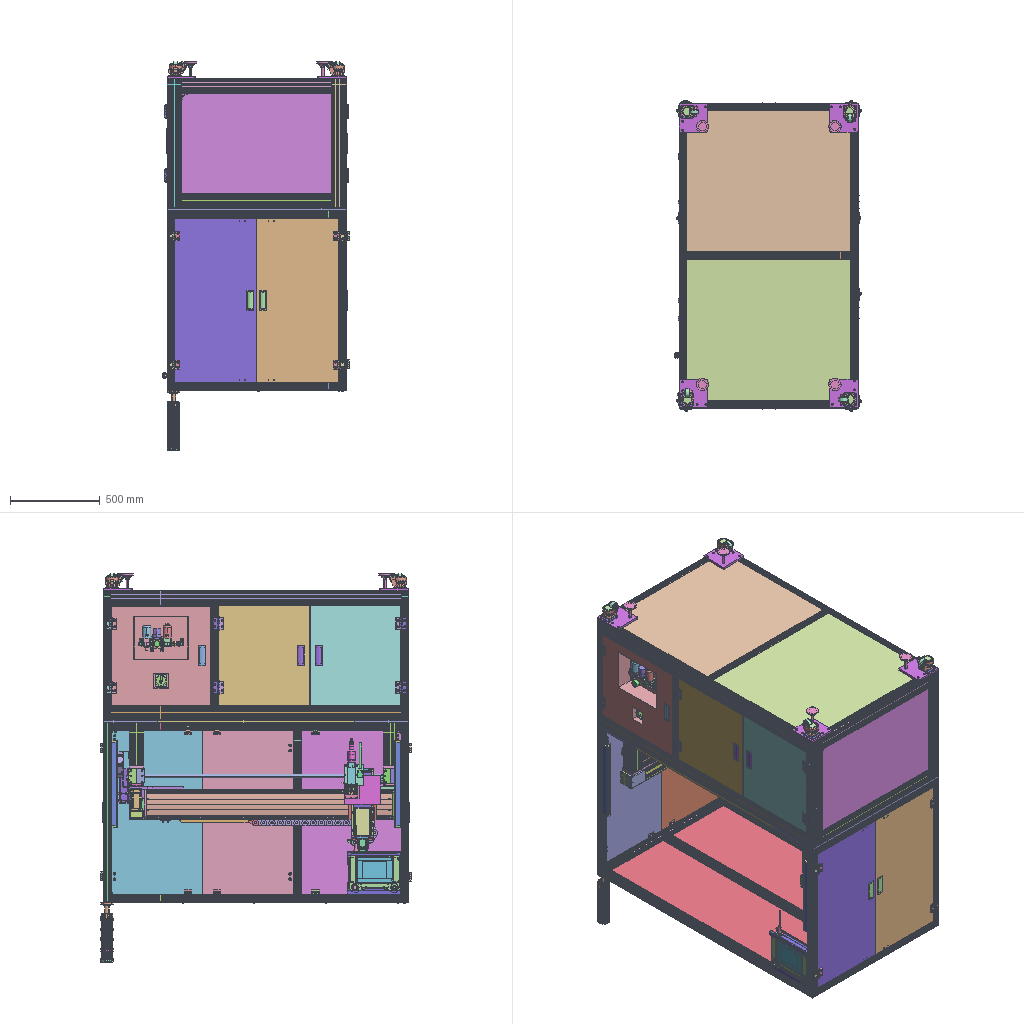Assembly | STEP file | 300 different items | 915 placed | box 1041 x 1735 x 2168 mm
Parts list (item | name | quantity | parent item | size | volume):
1 | 10B | x1 | in 20201224-195616-35202 | 290 x 230 x 35 mm | 178188 mm3
2 | 11B | x1 | in 20201224-195616-35202 | 290 x 385 x 37.5 mm | 218260 mm3
3 | 11M | x1 | in PLASMA | 71 x 79.5 x 170.1 mm | 187590 mm3
4 | 2 reset flat push button[GOB-2A10M-GW]_10M | x1 | in 2 reset flat push button[GOB-2A10M-GW]_GOB-2A10M-GW | 71 x 79.5 x 130.1 mm | 149787 mm3
5 | 82 fan grille | x1 | in Power supply model--JYDM(2)1 | 124.466 x 2.25 x 124.466 mm | 2127 mm3
6 | AC220V three-pin socket-KET-301 | x1 | in Power supply model--JYDM(2)1 | 50.485 x 22.8 x 28.4 mm | 5143 mm3
7 | AIR_PRESSURE_REGULATOR_SCREEN | x1 | in Power supply model--JYDM(2)1 | - | -
8 | AP0_ASM_ALL_SHEET_09 | x1 | in APO_ASM_SHEET_JYDM_WELDING_ASM | - | -
9 | AP0_ASM_ALL_SHEET_10 | x1 | in APO_ASM_SHEET_JYDM_WELDING_ASM | - | -
10 | AP0_ASM_ALL_SHEET_11 | x1 | in APO_ASM_SHEET_JYDM_WELDING_ASM | - | -
11 | AP0_ASM_JYDM_SHEET_04 | x1 | in Power supply model--JYDM(2)1 | 396.5 x 248 x 20 mm | 232744 mm3
12 | AP0_JYDM_SHEET_01 | x1 | in APO_ASM_SHEET_JYDM_WELDING_ASM | - | -
13 | AP0_JYDM_SHEET_02_05 | x1 | in APO_ASM_SHEET_JYDM_WELDING_ASM | - | -
14 | AP0_JYDM_SHEET_03 | x1 | in APO_ASM_SHEET_JYDM_WELDING_ASM | - | -
15 | AP0_JYDM_SHEET_07 | x1 | in Power supply model--JYDM(2)1 | 58 x 58 x 27.5 mm | 7319 mm3
16 | AP0_JYDM_SHEET_15 | x2 | in APO_ASM_SHEET_JYDM_WELDING_ASM | 20 x 13.5 x 70 mm | 4064 mm3
17 | B01-_X2_70B980F6_X0_ | x1 | in Standard three-color light | 68.5 x 68.5 x 39.5 mm | 31380 mm3
18 | Black terminal post | x1 | in Power supply model--JYDM(2)1 | 20.458 x 20.454 x 38 mm | 10782 mm3
19 | Blowing port | x1 | in Function head assembly | 19 x 192 x 30 mm | 38106 mm3
20 | CNTG-8 | x3 | in Power supply model--JYDM(2)1 | 38 x 22.2 x 22.2 mm | 6916 mm3
21 | Changeover switch LW30-63.... | x1 | in HJC0 frame | 65 x 65 x 101.647 mm | 216311 mm3
22 | FFH80-GY-002A^FFH85-B3 -02_three-axis module | x1 | in FFH85-B3 -02^three-axis module | 110 x 81 x 42.5 mm | 368601 mm3
23 | FFH80-GY-002A^FFH85-PL-M75-B3-01_three-axis module | x1 | in FFH85-PL-M75-B3-01^three-axis module | 110 x 81 x 42.5 mm | 368601 mm3
24 | FFH80-GY-002B^FFH85-B3 -02_three-axis module | x1 | in FFH85-B3 -02^three-axis module | 110 x 81 x 42.5 mm | 366642 mm3
25 | FFH80-GY-002B^FFH85-PL-M75-B3-01_three-axis module | x1 | in FFH85-PL-M75-B3-01^three-axis module | 110 x 81 x 42.5 mm | 366642 mm3
26 | FFH80-GY-003A^FFH85-PL-M75-B3-01_three-axis module | x1 | in FFH85-PL-M75-B3-01^three-axis module | 90 x 81 x 42.5 mm | 300723 mm3
27 | FFH80-GY-003B^FFH85-B3 -02_three-axis module | x1 | in FFH85-B3 -02^three-axis module | 90 x 81 x 42.5 mm | 303054 mm3
28 | FFH80-GY-003B^FFH85-PL-M75-B3-01_three-axis module | x1 | in FFH85-PL-M75-B3-01^three-axis module | 90 x 81 x 42.5 mm | 303221 mm3
29 | FFH80-GY-004^FFH85-B3 -02_three-axis module | x1 | in FFH85-B3 -02^three-axis module | 78 x 17.5 x 210 mm | 184560 mm3
30 | FFH80-GY-004^FFH85-PL-M75-B3-01_three-axis module | x1 | in FFH85-PL-M75-B3-01^three-axis module | 78 x 17.5 x 210 mm | 184560 mm3
31 | FFH80-GY-007^FFH85-PL-M75-B3-01_three-axis module | x1 | in FFH85-PL-M75-B3-01^three-axis module | 16.7 x 71.8 x 210 mm | 16698 mm3
32 | FFH80-GY-019^FFH85-B3 -02_three-axis module | x1 | in FFH85-B3 -02^three-axis module | 11 x 32.5 x 30 mm | 540.052 mm3
33 | FFH80-GY-020^FFH85-B3 -02_three-axis module | x1 | in FFH85-B3 -02^three-axis module | 1 x 12 x 52 mm | 601.324 mm3
34 | FFH80-GY-020^FFH85-PL-M75-B3-01_three-axis module | x1 | in FFH85-PL-M75-B3-01^three-axis module | 1 x 12 x 52 mm | 601.324 mm3
35 | FFH80-GY-022^FFH85-B3 -02_three-axis module | x1 | in FFH85-B3 -02^three-axis module | 1 x 60 x 60 mm | 3497 mm3
36 | FFH80-GY-022^FFH85-PL-M75-B3-01_three-axis module | x1 | in FFH85-PL-M75-B3-01^three-axis module | 1 x 60 x 60 mm | 3183 mm3
37 | FFH80-PL-008^FFH85-PL-M75-B3-01_three-axis module | x1 | in FFH85-PL-M75-B3-01^three-axis module | 10 x 81 x 192 mm | 99409 mm3
38 | FFH80-PL-018^FFH85-PL-M75-B3-01_three-axis module | x1 | in FFH85-PL-M75-B3-01^three-axis module | 40 x 81 x 192 mm | 36491 mm3
39 | FFH85-PL-011^FFH85-B3 -02_three-axis module | x1 | in FFH85-B3 -02^three-axis module | 85 x 81.5 x 722 mm | 4571503 mm3
40 | FFH85-PL-011^FFH85-PL-M75-B3-01_three-axis module | x1 | in FFH85-PL-M75-B3-01^three-axis module | 85 x 81.5 x 722 mm | 4571503 mm3
41 | LES120 base^FTH120-PD-direct-drive motor | x1 | in FTH120-PD-direct-drive motor | 120 x 58.2 x 361 mm | 888323 mm3
42 | LES120 bearing housing^FTH120-PD-direct-drive motor | x1 | in FTH120-PD-direct-drive motor | 119 x 56.7 x 13 mm | 72115 mm3
43 | LES120 direct-drive module^FTH120-PD-direct-drive motor | x1 | in FTH120-PD-direct-drive motor | - | -
44 | LES120 front cover^FTH120-PD-direct-drive motor | x1 | in FTH120-PD-direct-drive motor | 119 x 56.7 x 15 mm | 90652 mm3
45 | LES120 homing stopper^FTH120-PD-direct-drive motor | x1 | in FTH120-PD-direct-drive motor | 15 x 17.5 x 1 mm | 238.966 mm3
46 | LES120 slide base^FTH120-PD-direct-drive motor | x1 | in FTH120-PD-direct-drive motor | 115 x 18.873 x 108 mm | 136774 mm3
47 | LES120 steel strip pressure plate^FTH120-PD-direct-drive motor | x2 | in FTH120-PD-direct-drive motor | 87 x 10 x 1 mm | 849.899 mm3
48 | LES120 steel strip^FTH120-PD-direct-drive motor | x1 | in FTH120-PD-direct-drive motor | 385.8 x 0.15 x 86 mm | 4964 mm3
49 | LES120 top cover^FTH120-PD-direct-drive motor | x1 | in FTH120-PD-direct-drive motor | 201 x 16.2 x 118 mm | 41250 mm3
50 | M6 grease nipple^FTH120-PD-direct-drive motor | x2 | in FTH120-PD-direct-drive motor | 6.928 x 8 x 13.96 mm | 368.725 mm3
51 | M75^FFH85-PL-M75-B3-01_three-axis module | x1 | in FFH85-PL-M75-B3-01^three-axis module | - | -
52 | aaPT-T44^FFH85-B3 -02_three-axis module | x3 | in FFH85-B3 -02^three-axis module | 26 x 33.2 x 13.4 mm | 2334 mm3
53 | adapter plate^three-axis module | x1 | in 三轴模组-500-1000-150-20KG-B3(1) | 152 x 400 x 15 mm | 799832 mm3
54 | left limit^FTH120-PD-direct-drive motor | x1 | in FTH120-PD-direct-drive motor | - | -
55 | output terminal base plate^spray gun PTFE model | x1 | in Spray gun PTFE model | 90 x 90 x 3 mm | 23634 mm3
56 | output terminal cover plate^spray gun PTFE model | x1 | in Spray gun PTFE model | 63.5 x 63.5 x 20 mm | 34764 mm3
57 | output terminal^spray gun PTFE model | x1 | in Spray gun PTFE model | 63.5 x 63.5 x 35 mm | 72808 mm3
58 | DX-300 | x1 | in HJC1 frame | 61 x 240 x 300 mm | 251814 mm3
59 | Delta 400W servo motor ECMA-CX0604ES | x1 | in FTH120-PD-direct-drive motor | 94.241 x 160.702 x 147.367 mm | 450484 mm3
60 | Electrical board | x1 | in Back panel bracket | 15 x 460 x 1200 mm | 1154703 mm3
61 | Foot pad | x4 | in Power supply model--JYDM(2)1 | 20 x 20 x 10 mm | 3016 mm3
62 | HANDLE_130-91 | x1 | in Power supply model--JYDM(2)1 | 131 x 91 x 19.5 mm | 83642 mm3
63 | HJ60 Fuma caster mounting plate -A0 | x4 | in HJ60 Fuma caster foot assembly | 160 x 160 x 14 mm | 352458 mm3
64 | HJDX-000 | x1 | in Function head assembly | 200 x 16 x 160 mm | 512000 mm3
65 | HJDX-002 | x1 | in Function head assembly | 12 x 120 x 110 mm | 152611 mm3
66 | HJDX-003 | x1 | in Function head assembly | 12 x 120 x 76 mm | 105432 mm3
67 | HJDX-007 | x2 | in Bracket assembly | 16 x 80 x 900 mm | 1151503 mm3
68 | HJDX-008 | x4 | in HJC0 frame | 18 x 46 x 16 mm | 5416 mm3
69 | HJDX-200 | x2 | in HJC0 frame | 16 x 1000 x 300 mm | 4799343 mm3
70 | HJDX-201 | x1 | in 三轴模组-500-1000-150-20KG-B3(1) | 185 x 210 x 300 mm | 1834119 mm3
71 | HJDX-202 | x1 | in 三轴模组-500-1000-150-20KG-B3(1) | 185 x 210 x 300 mm | 1834119 mm3
72 | HJDX-203 | x1 | in HJC0 frame | 16 x 1100 x 240 mm | 4223323 mm3
73 | HJDX-204 | x1 | in HJC0 frame | 16 x 1100 x 160 mm | 2815363 mm3
74 | HJDX-300 | x1 | in 三轴模组-500-1000-150-20KG-B3(1) | 40 x 110 x 700 mm | 173965 mm3
75 | HJDX-301 | x1 | in 三轴模组-500-1000-150-20KG-B3(1) | 63.5 x 100 x 850 mm | 205101 mm3
76 | HJDX-302 | x1 | in 三轴模组-500-1000-150-20KG-B3(1) | 60 x 60 x 200 mm | 78199 mm3
77 | HJDX-303 | x1 | in 三轴模组-500-1000-150-20KG-B3(1) | 40 x 103 x 160 mm | 40590 mm3
78 | HJDX-304 | x1 | in HJC0 frame | - | 1378157 mm3
79 | HJDX-305 | x1 | in HJC0 frame | 1220 x 680 x 110 mm | 1513964 mm3
80 | HJDX-306 | x1 | in HJC0 frame | 50 x 638 x 396 mm | 649767 mm3
81 | HJHI_CGR51-60-U-001 | x4 | in HJGD-60F Fuma caster_GD-60F | 28 x 49 x 49 mm | 43690 mm3
82 | HJHI_CGR51-60-U-002 | x4 | in HJGD-60F Fuma caster_GD-60F | 70 x 63 x 89.5 mm | 81661 mm3
83 | HJHI_CGR51-60-U-003 | x4 | in HJGD-60F Fuma caster_GD-60F | 73 x 29.8 x 73 mm | 47628 mm3
84 | HJHI_CGR51-60-U-004 | x4 | in HJGD-60F Fuma caster_GD-60F | 55 x 39.5 x 55 mm | 65698 mm3
85 | HJLE-8-4080-S-OO_LE0724151524 | x1 | in HJC0 frame | 80 x 40 x 840 mm | 675539 mm3
86 | HJLE-8-4080-S-OO_LE0724151617 | x1 | in HJC0 frame | 80 x 40 x 840 mm | 675539 mm3
87 | HJLE-8-4080-S-OO_LE0724151624 | x1 | in HJC0 frame | 80 x 40 x 840 mm | 675539 mm3
88 | HJLE-8-4080-S-OO_LE0724151632 | x1 | in HJC0 frame | 80 x 40 x 840 mm | 675539 mm3
89 | HJLE-8-4080-S-OO_LE0724151639 | x1 | in HJC0 frame | 80 x 40 x 1620 mm | 1302826 mm3
90 | HJLE-8-4080-S-OO_LE0724151648 | x1 | in HJC0 frame | 80 x 40 x 1620 mm | 1302826 mm3
91 | HJLE-8-4080-S-OO_LE0724152727 | x1 | in HJC0 frame | 80 x 40 x 1620 mm | 1302826 mm3
92 | HJLE-8-4080-S-OO_LE0724152736 | x1 | in HJC0 frame | 80 x 40 x 1620 mm | 1302826 mm3
93 | HJLE-JJ90°-40_LE0724153021 | x1 | in HJLE-JJ90°-40-SET_LE0724153021 | 32 x 35 x 35 mm | 12807 mm3
94 | HJLE-TXM-M8-40_LE0724153021 | x2 | in HJLE-JJ90°-40-SET_LE0724153021 | 13.848 x 23 x 8.25 mm | 1654 mm3
95 | HJLE-YZS-M8X16_LE0724153021 | x2 | in HJLE-JJ90°-40-SET_LE0724153021 | 13 x 13 x 24 mm | 1703 mm3
96 | HJM12-150 | x4 | in HJ60 Fuma caster foot assembly | 70 x 70 x 146 mm | 64178 mm3
97 | LAS1_AGQ_TS[LAS1_AGQ_TS]_LAS1_AGQ_TS | x1 | in 20201224-195616-35202 | 67 x 32 x 31.988 mm | 25923 mm3
98 | LE-8-4040-S-OO_LE0311094925 | x1 | in HJC1 frame | 40 x 40 x 1000 mm | 478249 mm3
99 | LE-8-4040-S-OO_LE0311094928 | x1 | in HJC1 frame | 40 x 40 x 1620 mm | 774763 mm3
100 | LE-8-4040-S-OO_LE0311094931 | x1 | in HJC1 frame | 40 x 40 x 920 mm | 439989 mm3
101 | LE-8-4040-S-OO_LE0311094933 | x1 | in HJC1 frame | 40 x 40 x 1620 mm | 774763 mm3
102 | LE-8-4040-S-OO_LE0311094936 | x1 | in HJC1 frame | 40 x 40 x 920 mm | 439989 mm3
103 | LE-8-4040-S-OO_LE0311094939 | x1 | in HJC1 frame | 40 x 40 x 1000 mm | 478249 mm3
104 | LE-8-4040-S-OO_LE0311094942 | x1 | in HJC1 frame | 40 x 40 x 1000 mm | 478249 mm3
105 | LE-8-4040-S-OO_LE0311094946 | x1 | in HJC1 frame | 40 x 40 x 1000 mm | 478249 mm3
106 | LE-8-4040-S-OO_LE0311094949 | x1 | in HJC1 frame | 40 x 40 x 920 mm | 439466 mm3
107 | LE-8-4040-S-OO_LE0311094953 | x1 | in HJC1 frame | 40 x 40 x 1620 mm | 773979 mm3
108 | LE-8-4040-S-OO_LE0311094956 | x1 | in HJC1 frame | 40 x 40 x 920 mm | 439466 mm3
109 | LE-8-4040-S-OO_LE0311095410 | x1 | in HJC1 frame | 40 x 40 x 1620 mm | 774763 mm3
110 | LE-8-4040-S-OO_LE0314001325 | x1 | in HJC0 frame | 40 x 40 x 560 mm | 267819 mm3
111 | LE-8-4040-S-OO_LE0314001329 | x1 | in HJC0 frame | 40 x 40 x 560 mm | 267819 mm3
112 | LE-8-4040-S-OO_LE0314010410 | x1 | in Back panel bracket | 40 x 40 x 1620 mm | 774763 mm3
113 | LE-8-4040-S-OO_LE0314010413 | x1 | in Back panel bracket | 40 x 40 x 1620 mm | 774763 mm3
114 | LE-8-4040-S-OO_LE0314010416 | x1 | in Back panel bracket | 40 x 40 x 320 mm | 153040 mm3
115 | LE-8-4040-S-OO_LE0314010419 | x1 | in Back panel bracket | 40 x 40 x 320 mm | 153040 mm3
116 | LE-8-4040-S-OO_LE0314010425 | x1 | in Back panel bracket | 40 x 40 x 320 mm | 153040 mm3
117 | LE-8-4040-S-OO_LE0314010428 | x1 | in Back panel bracket | 40 x 40 x 480 mm | 229559 mm3
118 | LE-8-4040-S-OO_LE0314010440 | x1 | in Back panel bracket | 40 x 40 x 480 mm | 229559 mm3
119 | LE-8-4040-S-OO_LE0314010444 | x1 | in Back panel bracket | 40 x 40 x 480 mm | 229559 mm3
120 | LE-8-4040-S-OO_LE0314011714 | x1 | in HJC0 frame | 40 x 40 x 920 mm | 439989 mm3
121 | LE-8-4040-S-OO_LE0314012646 | x1 | in HJC1 frame | 40 x 40 x 920 mm | 439989 mm3
122 | LE-8-4040-S-OO_LE0314180216 | x1 | in HJC0 frame | 40 x 40 x 1060 mm | 506943 mm3
123 | LE-8-4040-S-OO_LE0314180221 | x1 | in HJC0 frame | 40 x 40 x 1060 mm | 506943 mm3
124 | LE-8-4040-S-OO_LE0314200037 | x1 | in HJC0 frame | 40 x 40 x 600 mm | 286949 mm3
125 | LE-8-4040-S-OO_LE0314200041 | x1 | in HJC0 frame | 40 x 40 x 600 mm | 286949 mm3
126 | LE-8-4080-S-OO_LE0307101811 | x1 | in HJC0 frame | 80 x 40 x 720 mm | 579034 mm3
127 | LE-8-4080-S-OO_LE0307101836 | x1 | in HJC0 frame | 80 x 40 x 720 mm | 579034 mm3
128 | LE-8-4080-S-OO_LE0307101856 | x1 | in HJC0 frame | 80 x 40 x 720 mm | 579034 mm3
129 | LE-8-4080-S-OO_LE0307101920 | x1 | in HJC0 frame | 80 x 40 x 720 mm | 579034 mm3
130 | LE-8-4080-S-OO_LE0313224044 | x1 | in HJC0 frame | 80 x 40 x 920 mm | 739877 mm3
131 | LE-8-4080-S-OO_LE0313224113 | x1 | in HJC0 frame | 80 x 40 x 920 mm | 739877 mm3
132 | LE-8-8080-S-OO_LE0313205357 | x2 | in Bracket assembly | 80 x 80 x 740 mm | 1300909 mm3
133 | LE-8-8080-S-OO_LE0313205421 | x2 | in Bracket assembly | 80 x 80 x 240 mm | 421917 mm3
134 | LE-8-8080-S-OO_LE0313205425 | x2 | in Bracket assembly | 80 x 80 x 240 mm | 421917 mm3
135 | LE-BYS-M6X16_PN_0013 | x16 | in Flat sealing plate assembly_PN_0013 | 10.5 x 10.5 x 19.3 mm | 623.238 mm3
136 | LE-FL-M6_LE0314002639 | x4 | in LE-LHY-40A-SET_LE0314002639 | 14.2 x 14.2 x 6 mm | 478.178 mm3
137 | LE-FL-M6_LE0314012955 | x8 | in LE-NHY-40-SET_LE0314012955 | 14.2 x 14.2 x 6 mm | 478.178 mm3
138 | LE-FL-M6_PN_0002 | x8 | in LE-NHY-40-SET_LE0314012858 | 14.2 x 14.2 x 6 mm | 478.178 mm3
139 | LE-FL-M6_PN_0003 | x8 | in LE-LHY-40A-SET_LE0314002343 | 14.2 x 14.2 x 6 mm | 478.178 mm3
140 | LE-FL-M6_PN_0004 | x8 | in LE-LHY-40A-SET_LE0314002730 | 14.2 x 14.2 x 6 mm | 478.178 mm3
141 | LE-FL-M6_PN_0005 | x4 | in LE-LHY-40A-SET_LE0307104148 | 14.2 x 14.2 x 6 mm | 478.178 mm3
142 | LE-FL-M6_PN_0006 | x4 | in LE-NHY-40-SET_LE0314013112 | 14.2 x 14.2 x 6 mm | 478.178 mm3
143 | LE-FL-M6_PN_0009 | x8 | in LE-NHY-40-SET_LE0314013317 | 14.2 x 14.2 x 6 mm | 478.178 mm3
144 | LE-FL-M8_LE0314201254 | x12 | in Sheet-metal sealing plate assembly_PN_0011 | 17.9 x 17.9 x 8 mm | 1002 mm3
145 | LE-FL-M8_PN_0001 | x10 | in Sheet-metal sealing plate assembly_PN_0001 | 17.9 x 17.9 x 8 mm | 1002 mm3
146 | LE-FL-M8_PN_0008 | x12 | in Sheet-metal sealing plate assembly_PN_0008 | 17.9 x 17.9 x 8 mm | 1002 mm3
147 | LE-FL-M8_PN_0012 | x10 | in Sheet-metal sealing plate assembly_PN_0012 | 17.9 x 17.9 x 8 mm | 1002 mm3
148 | LE-LHY-40A_LE0307104148 | x2 | in LE-LHY-40A-SET_LE0307104148 | 58.5 x 74 x 15 mm | 28707 mm3
149 | LE-LHY-40A_LE0314002343 | x4 | in LE-LHY-40A-SET_LE0314002343 | 58.5 x 74 x 15 mm | 28707 mm3
150 | LE-LHY-40A_LE0314002639 | x2 | in LE-LHY-40A-SET_LE0314002639 | 58.5 x 74 x 15 mm | 28707 mm3
151 | LE-LHY-40A_LE0314002730 | x4 | in LE-LHY-40A-SET_LE0314002730 | 58.5 x 74 x 15 mm | 28707 mm3
152 | LE-LLS-96A_LE0307104148 | x1 | in LE-LLS-96A-SET_LE0307104148 | 110 x 18.2 x 38.5 mm | 52750 mm3
153 | LE-LLS-96A_LE0314002343 | x2 | in LE-LLS-96A-SET_LE0314002343 | 110 x 18.2 x 38.5 mm | 52750 mm3
154 | LE-LLS-96A_LE0314002639 | x1 | in LE-LLS-96A-SET_LE0314002639 | 110 x 18.2 x 38.5 mm | 52750 mm3
155 | LE-LLS-96A_LE0314002730 | x2 | in LE-LLS-96A-SET_LE0314002730 | 110 x 18.2 x 38.5 mm | 52750 mm3
156 | LE-LLS-96B_LE0314012858 | x2 | in LE-LLS-96B-SET_LE0314012858 | 112 x 18.2 x 38.5 mm | 54842 mm3
157 | LE-LLS-96B_LE0314012955 | x2 | in LE-LLS-96B-SET_LE0314012955 | 112 x 18.2 x 38.5 mm | 54842 mm3
158 | LE-LLS-96B_LE0314013112 | x1 | in LE-LLS-96B-SET_LE0314013112 | 112 x 18.2 x 38.5 mm | 54842 mm3
159 | LE-LLS-96B_LE0314013317 | x2 | in LE-LLS-96B-SET_LE0314013317 | 112 x 18.2 x 38.5 mm | 54842 mm3
160 | LE-MX-A-N_LE0307104148 | x4 | in LE-MX-A_PN_0005 | 11.547 x 10 x 3.2 mm | 207.255 mm3
161 | LE-MX-A-N_PN_0002 | x8 | in LE-MX-A_PN_0002 | 11.547 x 10 x 3.2 mm | 207.255 mm3
162 | LE-MX-A-N_PN_0003 | x8 | in LE-MX-A_PN_0003 | 11.547 x 10 x 3.2 mm | 207.255 mm3
163 | LE-MX-A-N_PN_0004 | x8 | in LE-MX-A_PN_0004 | 11.547 x 10 x 3.2 mm | 207.255 mm3
164 | LE-MX-A-N_PN_0006 | x4 | in LE-MX-A_LE0314013112 | 11.547 x 10 x 3.2 mm | 207.255 mm3
165 | LE-MX-A-N_PN_0007 | x8 | in LE-MX-A_PN_0007 | 11.547 x 10 x 3.2 mm | 207.255 mm3
166 | LE-MX-A-N_PN_0009 | x8 | in LE-MX-A_PN_0009 | 11.547 x 10 x 3.2 mm | 207.255 mm3
167 | LE-MX-A-N_PN_0010 | x4 | in LE-MX-A_PN_0010 | 11.547 x 10 x 3.2 mm | 207.255 mm3
168 | LE-MX-A-P1_LE0314002343 | x4 | in LE-MX-A_PN_0003 | 40 x 47.5 x 2 mm | 2610 mm3
169 | LE-MX-A-P1_LE0314002730 | x4 | in LE-MX-A_PN_0004 | 40 x 47.5 x 2 mm | 2610 mm3
170 | LE-MX-A-P1_PN_0002 | x4 | in LE-MX-A_PN_0002 | 40 x 47.5 x 2 mm | 2610 mm3
171 | LE-MX-A-P1_PN_0005 | x2 | in LE-MX-A_PN_0005 | 40 x 47.5 x 2 mm | 2610 mm3
172 | LE-MX-A-P1_PN_0006 | x2 | in LE-MX-A_LE0314013112 | 40 x 47.5 x 2 mm | 2610 mm3
173 | LE-MX-A-P1_PN_0007 | x4 | in LE-MX-A_PN_0007 | 40 x 47.5 x 2 mm | 2610 mm3
174 | LE-MX-A-P1_PN_0009 | x4 | in LE-MX-A_PN_0009 | 40 x 47.5 x 2 mm | 2610 mm3
175 | LE-MX-A-P1_PN_0010 | x2 | in LE-MX-A_PN_0010 | 40 x 47.5 x 2 mm | 2610 mm3
176 | LE-MX-A-P2_LE0314013112 | x2 | in LE-MX-A_LE0314013112 | 23 x 40 x 1.5 mm | 1331 mm3
177 | LE-MX-A-P2_PN_0002 | x4 | in LE-MX-A_PN_0002 | 23 x 40 x 1.5 mm | 1331 mm3
178 | LE-MX-A-P2_PN_0007 | x4 | in LE-MX-A_PN_0007 | 23 x 40 x 1.5 mm | 1331 mm3
179 | LE-MX-A-P2_PN_0009 | x4 | in LE-MX-A_PN_0009 | 23 x 40 x 1.5 mm | 1331 mm3
180 | LE-MX-A-TJG_LE0314002730 | x4 | in LE-MX-A_PN_0004 | 13 x 13 x 37 mm | 2296 mm3
181 | LE-MX-A-TJG_PN_0002 | x4 | in LE-MX-A_PN_0002 | 13 x 13 x 37 mm | 2296 mm3
182 | LE-MX-A-TJG_PN_0003 | x4 | in LE-MX-A_PN_0003 | 13 x 13 x 37 mm | 2296 mm3
183 | LE-MX-A-TJG_PN_0005 | x2 | in LE-MX-A_PN_0005 | 13 x 13 x 37 mm | 2296 mm3
184 | LE-MX-A-TJG_PN_0006 | x2 | in LE-MX-A_LE0314013112 | 13 x 13 x 37 mm | 2296 mm3
185 | LE-MX-A-TJG_PN_0007 | x4 | in LE-MX-A_PN_0007 | 13 x 13 x 37 mm | 2296 mm3
186 | LE-MX-A-TJG_PN_0009 | x4 | in LE-MX-A_PN_0009 | 13 x 13 x 37 mm | 2296 mm3
187 | LE-MX-A-TJG_PN_0010 | x2 | in LE-MX-A_PN_0010 | 13 x 13 x 37 mm | 2296 mm3
188 | LE-NHY-40_LE0314012858 | x4 | in LE-NHY-40-SET_LE0314012858 | 60 x 50 x 17 mm | 27546 mm3
189 | LE-NHY-40_LE0314012955 | x4 | in LE-NHY-40-SET_LE0314012955 | 60 x 50 x 17 mm | 27546 mm3
190 | LE-NHY-40_LE0314013112 | x2 | in LE-NHY-40-SET_LE0314013112 | 60 x 50 x 17 mm | 27546 mm3
191 | LE-NHY-40_LE0314013317 | x4 | in LE-NHY-40-SET_LE0314013317 | 60 x 50 x 17 mm | 27546 mm3
192 | LE-PJS-M6X12_LE0314012858 | x8 | in LE-NHY-40-SET_LE0314012858 | 12 x 12 x 12 mm | 458.016 mm3
193 | LE-PJS-M6X12_LE0314012955 | x8 | in LE-NHY-40-SET_LE0314012955 | 12 x 12 x 12 mm | 458.016 mm3
194 | LE-PJS-M6X12_PN_0006 | x4 | in LE-NHY-40-SET_LE0314013112 | 12 x 12 x 12 mm | 458.016 mm3
195 | LE-PJS-M6X12_PN_0009 | x8 | in LE-NHY-40-SET_LE0314013317 | 12 x 12 x 12 mm | 458.016 mm3
196 | LE-PJS-M6X16_PN_0003 | x16 | in LE-LHY-40A-SET_LE0314002343 | 12 x 12 x 16 mm | 571.113 mm3
197 | LE-PJS-M6X16_PN_0004 | x16 | in LE-LHY-40A-SET_LE0314002730 | 12 x 12 x 16 mm | 571.113 mm3
198 | LE-PJS-M6X16_PN_0005 | x8 | in LE-LHY-40A-SET_LE0307104148 | 12 x 12 x 16 mm | 571.113 mm3
199 | LE-PJS-M6X16_PN_0010 | x8 | in LE-LHY-40A-SET_LE0314002639 | 12 x 12 x 16 mm | 571.113 mm3
200 | LE-PJS-M6X25_PN_0002 | x8 | in LE-NHY-40-SET_LE0314012858 | 12 x 12 x 25 mm | 825.582 mm3
201 | LE-PJS-M6X25_PN_0006 | x4 | in LE-NHY-40-SET_LE0314013112 | 12 x 12 x 25 mm | 825.582 mm3
202 | LE-PJS-M6X25_PN_0007 | x8 | in LE-NHY-40-SET_LE0314012955 | 12 x 12 x 25 mm | 825.582 mm3
203 | LE-PJS-M6X25_PN_0009 | x8 | in LE-NHY-40-SET_LE0314013317 | 12 x 12 x 25 mm | 825.582 mm3
204 | LE-TM-M6-40_LE0307104148 | x8 | in LE-LHY-40A-SET_LE0307104148, LE-MX-A-SET_PN_0005 | 19.5 x 8 x 7.5 mm | 669.792 mm3
205 | LE-TM-M6-40_LE0314002730 | x16 | in LE-LHY-40A-SET_LE0314002730, LE-MX-A-SET_PN_0004 | 19.5 x 8 x 7.5 mm | 669.792 mm3
206 | LE-TM-M6-40_LE0314012858 | x16 | in LE-MX-A-SET_LE0314012858, LE-NHY-40-SET_LE0314012858 | 19.5 x 8 x 7.5 mm | 669.792 mm3
207 | LE-TM-M6-40_LE0314013532 | x16 | in Flat sealing plate assembly_PN_0013 | 19.5 x 8 x 7.5 mm | 669.792 mm3
208 | LE-TM-M6-40_PN_0003 | x16 | in LE-LHY-40A-SET_LE0314002343, LE-MX-A-SET_PN_0003 | 19.5 x 8 x 7.5 mm | 669.792 mm3
209 | LE-TM-M6-40_PN_0006 | x8 | in LE-MX-A-SET_LE0314013112, LE-NHY-40-SET_LE0314013112 | 19.5 x 8 x 7.5 mm | 669.792 mm3
210 | LE-TM-M6-40_PN_0007 | x16 | in LE-MX-A-SET_PN_0007, LE-NHY-40-SET_LE0314012955 | 19.5 x 8 x 7.5 mm | 669.792 mm3
211 | LE-TM-M6-40_PN_0009 | x16 | in LE-MX-A-SET_PN_0009, LE-NHY-40-SET_LE0314013317 | 19.5 x 8 x 7.5 mm | 669.792 mm3
212 | LE-TM-M6-40_PN_0010 | x8 | in LE-LHY-40A-SET_LE0314002639, LE-MX-A-SET_LE0314002639 | 19.5 x 8 x 7.5 mm | 669.792 mm3
213 | LE-TS-M8X16-40_LE0314002452 | x10 | in Sheet-metal sealing plate assembly_PN_0012 | 18 x 8 x 21.5 mm | 1450 mm3
214 | LE-TS-M8X16-40_PN_0001 | x10 | in Sheet-metal sealing plate assembly_PN_0001 | 18 x 8 x 21.5 mm | 1450 mm3
215 | LE-TS-M8X16-40_PN_0008 | x12 | in Sheet-metal sealing plate assembly_PN_0008 | 18 x 8 x 21.5 mm | 1450 mm3
216 | LE-TS-M8X16-40_PN_0011 | x12 | in Sheet-metal sealing plate assembly_PN_0011 | 18 x 8 x 21.5 mm | 1450 mm3
217 | LE-YZS-M4X10_PN_0002 | x8 | in LE-MX-A-SET_LE0314012858 | 7 x 7 x 14 mm | 258.83 mm3
218 | LE-YZS-M4X10_PN_0006 | x4 | in LE-MX-A-SET_LE0314013112 | 7 x 7 x 14 mm | 258.83 mm3
219 | LE-YZS-M4X10_PN_0007 | x8 | in LE-MX-A-SET_PN_0007 | 7 x 7 x 14 mm | 258.83 mm3
220 | LE-YZS-M4X10_PN_0009 | x8 | in LE-MX-A-SET_PN_0009 | 7 x 7 x 14 mm | 258.83 mm3
221 | LE-YZS-M6X12_PN_0002 | x8 | in LE-MX-A-SET_LE0314012858 | 10 x 10 x 18 mm | 726.537 mm3
222 | LE-YZS-M6X12_PN_0003 | x8 | in LE-MX-A-SET_PN_0003 | 10 x 10 x 18 mm | 726.537 mm3
223 | LE-YZS-M6X12_PN_0004 | x8 | in LE-MX-A-SET_PN_0004 | 10 x 10 x 18 mm | 726.537 mm3
224 | LE-YZS-M6X12_PN_0005 | x4 | in LE-MX-A-SET_PN_0005 | 10 x 10 x 18 mm | 726.537 mm3
225 | LE-YZS-M6X12_PN_0006 | x4 | in LE-MX-A-SET_LE0314013112 | 10 x 10 x 18 mm | 726.537 mm3
226 | LE-YZS-M6X12_PN_0007 | x8 | in LE-MX-A-SET_PN_0007 | 10 x 10 x 18 mm | 726.537 mm3
227 | LE-YZS-M6X12_PN_0009 | x8 | in LE-MX-A-SET_PN_0009 | 10 x 10 x 18 mm | 726.537 mm3
228 | LE-YZS-M6X12_PN_0010 | x4 | in LE-MX-A-SET_LE0314002639 | 10 x 10 x 18 mm | 726.537 mm3
229 | Left door panel sheet metal_PN_0003 | x1 | in Sheet-metal door assembly_PN_0003 | 508.5 x 557 x 15 mm | 531244 mm3
230 | Left door panel sheet metal_PN_0004 | x1 | in Sheet-metal door assembly_PN_0004 | 508.5 x 557 x 15 mm | 531244 mm3
231 | Left door panel sheet metal_PN_0010 | x1 | in Sheet-metal door assembly_PN_0010 | 558 x 557 x 15 mm | 577988 mm3
232 | Left door panel_PN_0002 | x1 | in Glass door assembly_PN_0002 | 458.5 x 917 x 8 mm | 3334170 mm3
233 | Left door panel_PN_0007 | x1 | in Glass door assembly_PN_0007 | 508.5 x 917 x 8 mm | 3700970 mm3
234 | Left door panel_PN_0009 | x1 | in Glass door assembly_PN_0009 | 458.5 x 917 x 8 mm | 3334170 mm3
235 | Light grating 20-22 | x2 | in HJC1 frame | 30 x 35 x 536 mm | 422875 mm3
236 | MAIN_SWITCH_KNOB | x1 | in Power supply model--JYDM(2)1 | 28 x 38.5 x 30 mm | 14086 mm3
237 | MT6070iH5[MT6070iH5]_MT6070iH5 | x1 | in 20201224-195616-35202 | 34 x 146.5 x 200.4 mm | 782719 mm3
238 | PH802. | x2 | in AC30-02G-A_0_ | 37.083 x 28 x 17.166 mm | 6341 mm3
239 | PLASMA_KNOB_SIZE | x1 | in Power supply model--JYDM(2)1 | 30.4 x 20 x 30.4 mm | 14168 mm3
240 | PRT0001-_X2_70B980F6_X0_ | x1 | in Standard three-color light | - | -
241 | Part 3^three-axis module | x1 | in 三轴模组-500-1000-150-20KG-B3(1) | 20 x 20 x 1337 mm | 420031 mm3
242 | Pneumatic circuit board | x1 | in Back panel bracket | 2 x 460 x 400 mm | 365879 mm3
243 | Right door panel sheet metal_PN_0003 | x1 | in Sheet-metal door assembly_PN_0003 | 508.5 x 557 x 15 mm | 531244 mm3
244 | Right door panel sheet metal_PN_0004 | x1 | in Sheet-metal door assembly_PN_0004 | 508.5 x 557 x 15 mm | 531244 mm3
245 | Right door panel sheet metal_PN_0005 | x1 | in 钣金DoorComponent_LE0307104148 | 558 x 557 x 103 mm | 763625 mm3
246 | Right door panel_PN_0002 | x1 | in Glass door assembly_PN_0002 | 458.5 x 917 x 8 mm | 3334170 mm3
247 | Right door panel_PN_0006 | x1 | in Glass door assembly_PN_0006 | 558 x 917 x 8 mm | 4064102 mm3
248 | Right door panel_PN_0007 | x1 | in Glass door assembly_PN_0007 | 508.5 x 917 x 8 mm | 3700970 mm3
249 | Right door panel_PN_0009 | x1 | in Glass door assembly_PN_0009 | 458.5 x 917 x 8 mm | 3334170 mm3
250 | Round selector switch[GQ115-C-11XA]_GQ115-C-11XA | x1 | in 20201224-195616-35202 | 18 x 47.347 x 18 mm | 5818 mm3
251 | SCREEN_JYDM | x1 | in Power supply model--JYDM(2)1 | - | -
252 | SRQ-FSK | x1 | in Power supply model--JYDM(2)1 | 92 x 92 x 25 mm | 27792 mm3
253 | Sheet-metal sealing plate_PN_0001 | x1 | in Sheet-metal sealing plate assembly_PN_0001 | 839 x 559 x 38 mm | 851235 mm3
254 | Sheet-metal sealing plate_PN_0008 | x1 | in Sheet-metal sealing plate assembly_PN_0008 | 919 x 789 x 38 mm | 1267247 mm3
255 | Sheet-metal sealing plate_PN_0011 | x1 | in Sheet-metal sealing plate assembly_PN_0011 | 919 x 789 x 38 mm | 1267247 mm3
256 | Sheet-metal sealing plate_PN_0012 | x1 | in Sheet-metal sealing plate assembly_PN_0012 | 839 x 559 x 38 mm | 851235 mm3
257 | TFH-CONNECTION57 | x36 | in 拖链-25系列全封闭两侧打开型 TFH25[TFH25-C57-R55-34]_TFH25-C57-R55-34 | 71 x 81 x 35 mm | 50324 mm3
258 | TFH-FIX-END57 | x2 | in 拖链-25系列全封闭两侧打开型 TFH25[TFH25-C57-R55-34]_TFH25-C57-R55-34 | 71 x 58.5 x 35 mm | 23684 mm3
259 | TFH-FREE-END57 | x2 | in 拖链-25系列全封闭两侧打开型 TFH25[TFH25-C57-R55-34]_TFH25-C57-R55-34 | 72 x 58.321 x 34.821 mm | 22010 mm3
260 | _AF30-02-A(0)_BODY | x1 | in AC30-02G-A_0_ | 53 x 45.8 x 53.4 mm | 97884 mm3
261 | _AF30-02-A_BOWL | x1 | in AC30-02G-A_0_ | 46 x 74.3 x 53 mm | 114802 mm3
262 | _AF30-A(0)_DRAIN | x1 | in AC30-02G-A_0_ | 19.5 x 11 x 8 mm | 1100 mm3
263 | _AL30-02-A(0)_BODY | x1 | in AC30-02G-A_0_ | 53 x 69.9 x 53.4 mm | 108117 mm3
264 | _AL30-A_BOWL | x1 | in AC30-02G-A_0_ | 46 x 74.3 x 53 mm | 115027 mm3
265 | _AR30-02G-A(0)_BODY | x1 | in AC30-02G-A_0_ | 53 x 48.5 x 57 mm | 90348 mm3
266 | _AR30-A_BONNET | x1 | in AC30-02G-A_0_ | 53 x 64.2 x 57 mm | 112882 mm3
267 | _AR30-G-A_GAUGE | x1 | in AC30-02G-A_0_ | 37.5 x 37.5 x 40.5 mm | 27726 mm3
268 | _HSV08 -slide.... | x1 | in HSV08.... | 30 x 30 x 32.5 mm | 8453 mm3
269 | _HSV08 Body.... | x1 | in HSV08.... | 21.939 x 19.4 x 58 mm | 11796 mm3
270 | _MXS-AS20-50AS_AOP-TM_1 | x1 | in MXS20-50ASP-M9NV_0_0_ | 21 x 13 x 25 mm | 6501 mm3
271 | _MXS-AS20_AOP-BM_1 | x1 | in MXS20-50ASP-M9NV_0_0_ | 24 x 45.5 x 27.5 mm | 15366 mm3
272 | _MXS20-50(0)_BODY_1 | x1 | in MXS20-50ASP-M9NV_0_0_ | 73 x 40 x 106.5 mm | 190258 mm3
273 | _MXS20-50ASP(0)_ROD | x1 | in MXS20-50ASP-M9NV_0_0_ | 76 x 46 x 121 mm | 178079 mm3
274 | _MXS20-50P(0)_FOP | x1 | in MXS20-50ASP-M9NV_0_0_ | 77.2 x 29 x 110 mm | 55359 mm3
275 | _MXS_D-M9NV(20)_1 | x2 | in MXS20-50ASP-M9NV_0_0_ | 4.6 x 21.5 x 20 mm | 612.131 mm3
276 | _Y300T-A_FRONT | x2 | in AC30-02G-A_0_ | 16.782 x 16 x 17.8 mm | 1225 mm3
277 | _Y300T-A_REAR | x2 | in AC30-02G-A_0_ | 19 x 82 x 28.6 mm | 16093 mm3
278 | _Y300T-A_SCREW | x2 | in AC30-02G-A_0_ | 7.2 x 43.4 x 43.1 mm | 7021 mm3
279 | - | x4 | in Standard three-color light | 70 x 65.6 x 70 mm | 40502 mm3
280 | - | x1 | in Standard three-color light | 70 x 16 x 70 mm | 11959 mm3
281 | 复件 400W^FHB175S-PRW-P40(马达RightUpper折-400W伺服电机) | x1 | in FHB175S-PRW-P40(马达RightUpper折-400W伺服电机) | - | -
282 | 复件 FFH80-GY-003A^复件 FFH85-B3 -02_三轴模组 | x1 | in FFH85-B3 -02^three-axis module | 90 x 81 x 42.5 mm | 300723 mm3
283 | 复件 FFH80-GY-007^复件 FFH85-B3 -02_三轴模组 | x1 | in FFH85-B3 -02^three-axis module | 16.7 x 71.8 x 210 mm | 16698 mm3
284 | 复件 FFH80-GY-019^复件 FFH85-PL-M75-B3-01_三轴模组 | x1 | in FFH85-PL-M75-B3-01^three-axis module | 11 x 32.5 x 30 mm | 540.052 mm3
285 | 复件 FHB175-001^FHB175S-PRW-P40(马达RightUpper折-400W伺服电机) | x1 | in FHB175S-PRW-P40(马达RightUpper折-400W伺服电机) | 170 x 102.4 x 10 mm | 124038 mm3
286 | 复件 FHB175-003^FHB175S-PRW-P40(马达RightUpper折-400W伺服电机) | x1 | in FHB175S-PRW-P40(马达RightUpper折-400W伺服电机) | 169 x 87 x 100.4 mm | 517435 mm3
287 | 复件 FHB175-004^FHB175S-PRW-P40(马达RightUpper折-400W伺服电机) | x1 | in FHB175S-PRW-P40(马达RightUpper折-400W伺服电机) | 169 x 49.5 x 152 mm | 495941 mm3
288 | 复件 FHB175-008^FHB175S-PRW-P40(马达RightUpper折-400W伺服电机) | x1 | in FHB175S-PRW-P40(马达RightUpper折-400W伺服电机) | 6 x 140.5 x 72 mm | 60684 mm3
289 | 复件 FHB175-012^FHB175S-PRW-P40(马达RightUpper折-400W伺服电机) | x1 | in FHB175S-PRW-P40(马达RightUpper折-400W伺服电机) | 30 x 60 x 8.3 mm | 863.995 mm3
290 | 复件 FHB175-018^FHB175S-PRW-P40(马达RightUpper折-400W伺服电机) | x1 | in FHB175S-PRW-P40(马达RightUpper折-400W伺服电机) | 140.5 x 72 x 39 mm | 25843 mm3
291 | 复件 FHB175-033^FHB175S-PRW-P40(马达RightUpper折-400W伺服电机) | x2 | in FHB175S-PRW-P40(马达RightUpper折-400W伺服电机) | 62 x 76 x 2 mm | 9274 mm3
292 | 复件 FHB175-034^FHB175S-PRW-P40(马达RightUpper折-400W伺服电机) | x1 | in FHB175S-PRW-P40(马达RightUpper折-400W伺服电机) | 62 x 62 x 8 mm | 29127 mm3
293 | 复件 FHB175-PRW-011^FHB175S-PRW-P40(马达RightUpper折-400W伺服电机) | x1 | in FHB175S-PRW-P40(马达RightUpper折-400W伺服电机) | 170 x 103.1 x 1372 mm | 11406722 mm3
294 | 复件 aaPT-T44^FHB175S-PRW-P40(马达RightUpper折-400W伺服电机) | x3 | in FHB175S-PRW-P40(马达RightUpper折-400W伺服电机) | 26 x 33.2 x 13.4 mm | 2334 mm3
295 | 复件 aaPT-T44^复件 FFH85-PL-M75-B3-01_三轴模组 | x3 | in FFH85-PL-M75-B3-01^three-axis module | 26 x 33.2 x 13.4 mm | 2334 mm3
296 | 复件 Right极限^FTH120-PD-马达直连 | x2 | in FTH120-PD-direct-drive motor | - | -
297 | 平铺封Plate_LE0314013532 | x1 | in Flat sealing plate assembly_PN_0013 | 1000 x 1700 x 5 mm | 8497328 mm3
298 | 标准常压直喷喷枪(常规)(1)(1) | x1 | in Function head assembly | - | -
299 | 航插-1 | x2 | in Aviation plug assembly | 21.708 x 18.872 x 20 mm | 2692 mm3
300 | 航插-2 | x2 | in Aviation plug assembly | 34.8 x 17.5 x 17.5 mm | 1736 mm3